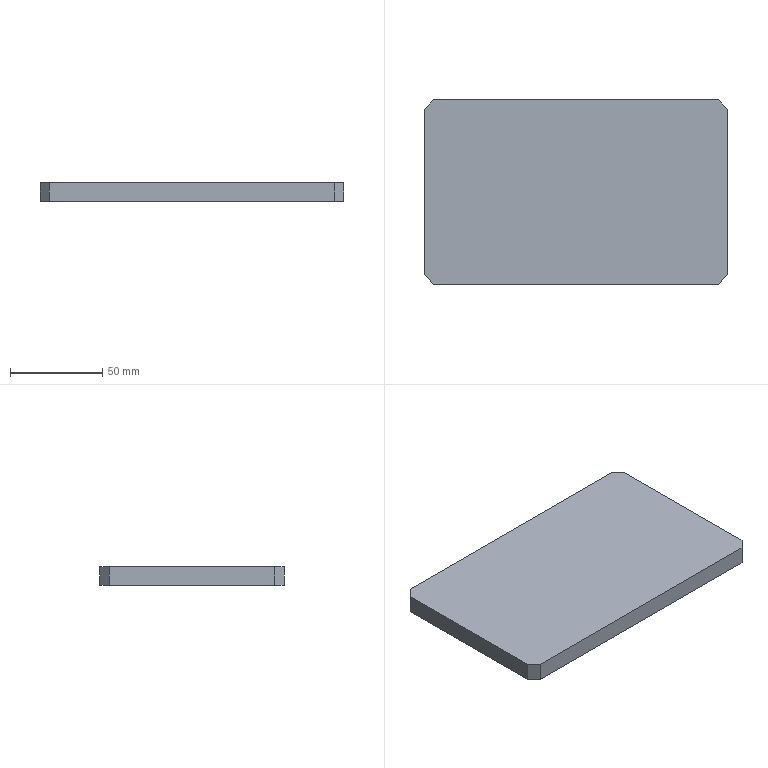Part | STEP file | Servo mount | 1 solid | 10 faces | box 165 x 100 x 10 mm | volume 164500 mm3 | plane 10
STEP:
#1=CARTESIAN_POINT('',(0.,0.,0.));
#2=DIRECTION('',(0.,0.,1.));
#3=DIRECTION('',(1.,0.,0.));
#4=AXIS2_PLACEMENT_3D('',#1,#2,#3);
#5=CARTESIAN_POINT('',(82.5,-45.,10.));
#6=VERTEX_POINT('',#5);
#7=CARTESIAN_POINT('',(82.5,45.,10.));
#8=VERTEX_POINT('',#7);
#9=CARTESIAN_POINT('',(82.5,50.,10.));
#10=DIRECTION('',(0.,1.,0.));
#11=VECTOR('',#10,1.);
#12=LINE('',#9,#11);
#13=CARTESIAN_POINT('',(82.5,50.,10.));
#14=DIRECTION('',(-1.,0.,0.));
#15=DIRECTION('',(0.,-1.,0.));
#16=AXIS2_PLACEMENT_3D('',#13,#14,#15);
#17=PLANE('',#16);
#18=CARTESIAN_POINT('',(0.,0.));
#19=DIRECTION('',(-1.,0.));
#20=VECTOR('',#19,1.);
#21=LINE('',#18,#20);
#22=(GEOMETRIC_REPRESENTATION_CONTEXT(2)PARAMETRIC_REPRESENTATION_CONTEXT()REPRESENTATION_CONTEXT('',''));
#23=DEFINITIONAL_REPRESENTATION('',(#21),#22);
#24=PCURVE('',#17,#23);
#25=CARTESIAN_POINT('',(82.5,-50.,10.));
#26=DIRECTION('',(0.,0.,1.));
#27=DIRECTION('',(1.,0.,0.));
#28=AXIS2_PLACEMENT_3D('',#25,#26,#27);
#29=PLANE('',#28);
#30=CARTESIAN_POINT('',(0.,100.));
#31=DIRECTION('',(0.,1.));
#32=VECTOR('',#31,1.);
#33=LINE('',#30,#32);
#34=(GEOMETRIC_REPRESENTATION_CONTEXT(2)PARAMETRIC_REPRESENTATION_CONTEXT()REPRESENTATION_CONTEXT('',''));
#35=DEFINITIONAL_REPRESENTATION('',(#33),#34);
#36=PCURVE('',#29,#35);
#37=SURFACE_CURVE('',#12,(#24,#36),.PCURVE_S1.);
#38=EDGE_CURVE('',#6,#8,#37,.T.);
#39=ORIENTED_EDGE('',*,*,#38,.F.);
#40=CARTESIAN_POINT('',(82.5,-45.,0.));
#41=VERTEX_POINT('',#40);
#42=CARTESIAN_POINT('',(82.5,-45.,10.));
#43=DIRECTION('',(0.,0.,-1.));
#44=VECTOR('',#43,1.);
#45=LINE('',#42,#44);
#46=CARTESIAN_POINT('',(95.,0.));
#47=DIRECTION('',(0.,-1.));
#48=VECTOR('',#47,1.);
#49=LINE('',#46,#48);
#50=(GEOMETRIC_REPRESENTATION_CONTEXT(2)PARAMETRIC_REPRESENTATION_CONTEXT()REPRESENTATION_CONTEXT('',''));
#51=DEFINITIONAL_REPRESENTATION('',(#49),#50);
#52=PCURVE('',#17,#51);
#53=CARTESIAN_POINT('',(82.5,-45.,10.));
#54=DIRECTION('',(-0.7071,0.7071,0.));
#55=DIRECTION('',(-0.7071,-0.7071,0.));
#56=AXIS2_PLACEMENT_3D('',#53,#54,#55);
#57=PLANE('',#56);
#58=CARTESIAN_POINT('',(0.,0.));
#59=DIRECTION('',(0.,-1.));
#60=VECTOR('',#59,1.);
#61=LINE('',#58,#60);
#62=(GEOMETRIC_REPRESENTATION_CONTEXT(2)PARAMETRIC_REPRESENTATION_CONTEXT()REPRESENTATION_CONTEXT('',''));
#63=DEFINITIONAL_REPRESENTATION('',(#61),#62);
#64=PCURVE('',#57,#63);
#65=SURFACE_CURVE('',#45,(#52,#64),.PCURVE_S1.);
#66=EDGE_CURVE('',#6,#41,#65,.T.);
#67=ORIENTED_EDGE('',*,*,#66,.T.);
#68=CARTESIAN_POINT('',(82.5,45.,0.));
#69=VERTEX_POINT('',#68);
#70=CARTESIAN_POINT('',(82.5,50.,0.));
#71=DIRECTION('',(0.,1.,0.));
#72=VECTOR('',#71,1.);
#73=LINE('',#70,#72);
#74=CARTESIAN_POINT('',(0.,-10.));
#75=DIRECTION('',(-1.,0.));
#76=VECTOR('',#75,1.);
#77=LINE('',#74,#76);
#78=(GEOMETRIC_REPRESENTATION_CONTEXT(2)PARAMETRIC_REPRESENTATION_CONTEXT()REPRESENTATION_CONTEXT('',''));
#79=DEFINITIONAL_REPRESENTATION('',(#77),#78);
#80=PCURVE('',#17,#79);
#81=CARTESIAN_POINT('',(82.5,-50.,0.));
#82=DIRECTION('',(0.,0.,1.));
#83=DIRECTION('',(1.,0.,0.));
#84=AXIS2_PLACEMENT_3D('',#81,#82,#83);
#85=PLANE('',#84);
#86=CARTESIAN_POINT('',(0.,100.));
#87=DIRECTION('',(0.,1.));
#88=VECTOR('',#87,1.);
#89=LINE('',#86,#88);
#90=(GEOMETRIC_REPRESENTATION_CONTEXT(2)PARAMETRIC_REPRESENTATION_CONTEXT()REPRESENTATION_CONTEXT('',''));
#91=DEFINITIONAL_REPRESENTATION('',(#89),#90);
#92=PCURVE('',#85,#91);
#93=SURFACE_CURVE('',#73,(#80,#92),.PCURVE_S1.);
#94=EDGE_CURVE('',#41,#69,#93,.T.);
#95=ORIENTED_EDGE('',*,*,#94,.T.);
#96=CARTESIAN_POINT('',(82.5,45.,10.));
#97=DIRECTION('',(0.,0.,1.));
#98=VECTOR('',#97,1.);
#99=LINE('',#96,#98);
#100=CARTESIAN_POINT('',(5.,0.));
#101=DIRECTION('',(0.,1.));
#102=VECTOR('',#101,1.);
#103=LINE('',#100,#102);
#104=(GEOMETRIC_REPRESENTATION_CONTEXT(2)PARAMETRIC_REPRESENTATION_CONTEXT()REPRESENTATION_CONTEXT('',''));
#105=DEFINITIONAL_REPRESENTATION('',(#103),#104);
#106=PCURVE('',#17,#105);
#107=CARTESIAN_POINT('',(77.5,50.,10.));
#108=DIRECTION('',(-0.7071,-0.7071,0.));
#109=DIRECTION('',(0.7071,-0.7071,0.));
#110=AXIS2_PLACEMENT_3D('',#107,#108,#109);
#111=PLANE('',#110);
#112=CARTESIAN_POINT('',(7.071,0.));
#113=DIRECTION('',(0.,1.));
#114=VECTOR('',#113,1.);
#115=LINE('',#112,#114);
#116=(GEOMETRIC_REPRESENTATION_CONTEXT(2)PARAMETRIC_REPRESENTATION_CONTEXT()REPRESENTATION_CONTEXT('',''));
#117=DEFINITIONAL_REPRESENTATION('',(#115),#116);
#118=PCURVE('',#111,#117);
#119=SURFACE_CURVE('',#99,(#106,#118),.PCURVE_S1.);
#120=EDGE_CURVE('',#69,#8,#119,.T.);
#121=ORIENTED_EDGE('',*,*,#120,.T.);
#122=EDGE_LOOP('',(#39,#67,#95,#121));
#123=FACE_BOUND('',#122,.T.);
#124=ADVANCED_FACE('',(#123),#17,.F.);
#125=CARTESIAN_POINT('',(77.5,50.,0.));
#126=VERTEX_POINT('',#125);
#127=CARTESIAN_POINT('',(-77.5,50.,0.));
#128=VERTEX_POINT('',#127);
#129=CARTESIAN_POINT('',(-82.5,50.,0.));
#130=DIRECTION('',(-1.,0.,0.));
#131=VECTOR('',#130,1.);
#132=LINE('',#129,#131);
#133=CARTESIAN_POINT('',(-82.5,50.,10.));
#134=DIRECTION('',(0.,-1.,0.));
#135=DIRECTION('',(0.,0.,-1.));
#136=AXIS2_PLACEMENT_3D('',#133,#134,#135);
#137=PLANE('',#136);
#138=CARTESIAN_POINT('',(10.,0.));
#139=DIRECTION('',(0.,-1.));
#140=VECTOR('',#139,1.);
#141=LINE('',#138,#140);
#142=(GEOMETRIC_REPRESENTATION_CONTEXT(2)PARAMETRIC_REPRESENTATION_CONTEXT()REPRESENTATION_CONTEXT('',''));
#143=DEFINITIONAL_REPRESENTATION('',(#141),#142);
#144=PCURVE('',#137,#143);
#145=CARTESIAN_POINT('',(-165.,100.));
#146=DIRECTION('',(-1.,0.));
#147=VECTOR('',#146,1.);
#148=LINE('',#145,#147);
#149=(GEOMETRIC_REPRESENTATION_CONTEXT(2)PARAMETRIC_REPRESENTATION_CONTEXT()REPRESENTATION_CONTEXT('',''));
#150=DEFINITIONAL_REPRESENTATION('',(#148),#149);
#151=PCURVE('',#85,#150);
#152=SURFACE_CURVE('',#132,(#144,#151),.PCURVE_S1.);
#153=EDGE_CURVE('',#126,#128,#152,.T.);
#154=ORIENTED_EDGE('',*,*,#153,.T.);
#155=CARTESIAN_POINT('',(-77.5,50.,10.));
#156=VERTEX_POINT('',#155);
#157=CARTESIAN_POINT('',(-77.5,50.,10.));
#158=DIRECTION('',(0.,0.,1.));
#159=VECTOR('',#158,1.);
#160=LINE('',#157,#159);
#161=CARTESIAN_POINT('',(0.,5.));
#162=DIRECTION('',(-1.,0.));
#163=VECTOR('',#162,1.);
#164=LINE('',#161,#163);
#165=(GEOMETRIC_REPRESENTATION_CONTEXT(2)PARAMETRIC_REPRESENTATION_CONTEXT()REPRESENTATION_CONTEXT('',''));
#166=DEFINITIONAL_REPRESENTATION('',(#164),#165);
#167=PCURVE('',#137,#166);
#168=CARTESIAN_POINT('',(-82.5,45.,10.));
#169=DIRECTION('',(0.7071,-0.7071,0.));
#170=DIRECTION('',(0.7071,0.7071,0.));
#171=AXIS2_PLACEMENT_3D('',#168,#169,#170);
#172=PLANE('',#171);
#173=CARTESIAN_POINT('',(7.071,0.));
#174=DIRECTION('',(0.,1.));
#175=VECTOR('',#174,1.);
#176=LINE('',#173,#175);
#177=(GEOMETRIC_REPRESENTATION_CONTEXT(2)PARAMETRIC_REPRESENTATION_CONTEXT()REPRESENTATION_CONTEXT('',''));
#178=DEFINITIONAL_REPRESENTATION('',(#176),#177);
#179=PCURVE('',#172,#178);
#180=SURFACE_CURVE('',#160,(#167,#179),.PCURVE_S1.);
#181=EDGE_CURVE('',#128,#156,#180,.T.);
#182=ORIENTED_EDGE('',*,*,#181,.T.);
#183=CARTESIAN_POINT('',(77.5,50.,10.));
#184=VERTEX_POINT('',#183);
#185=CARTESIAN_POINT('',(-82.5,50.,10.));
#186=DIRECTION('',(-1.,0.,0.));
#187=VECTOR('',#186,1.);
#188=LINE('',#185,#187);
#189=CARTESIAN_POINT('',(0.,0.));
#190=DIRECTION('',(0.,-1.));
#191=VECTOR('',#190,1.);
#192=LINE('',#189,#191);
#193=(GEOMETRIC_REPRESENTATION_CONTEXT(2)PARAMETRIC_REPRESENTATION_CONTEXT()REPRESENTATION_CONTEXT('',''));
#194=DEFINITIONAL_REPRESENTATION('',(#192),#193);
#195=PCURVE('',#137,#194);
#196=CARTESIAN_POINT('',(-165.,100.));
#197=DIRECTION('',(-1.,0.));
#198=VECTOR('',#197,1.);
#199=LINE('',#196,#198);
#200=(GEOMETRIC_REPRESENTATION_CONTEXT(2)PARAMETRIC_REPRESENTATION_CONTEXT()REPRESENTATION_CONTEXT('',''));
#201=DEFINITIONAL_REPRESENTATION('',(#199),#200);
#202=PCURVE('',#29,#201);
#203=SURFACE_CURVE('',#188,(#195,#202),.PCURVE_S1.);
#204=EDGE_CURVE('',#184,#156,#203,.T.);
#205=ORIENTED_EDGE('',*,*,#204,.F.);
#206=CARTESIAN_POINT('',(77.5,50.,10.));
#207=DIRECTION('',(0.,0.,-1.));
#208=VECTOR('',#207,1.);
#209=LINE('',#206,#208);
#210=CARTESIAN_POINT('',(0.,160.));
#211=DIRECTION('',(1.,0.));
#212=VECTOR('',#211,1.);
#213=LINE('',#210,#212);
#214=(GEOMETRIC_REPRESENTATION_CONTEXT(2)PARAMETRIC_REPRESENTATION_CONTEXT()REPRESENTATION_CONTEXT('',''));
#215=DEFINITIONAL_REPRESENTATION('',(#213),#214);
#216=PCURVE('',#137,#215);
#217=CARTESIAN_POINT('',(0.,0.));
#218=DIRECTION('',(0.,-1.));
#219=VECTOR('',#218,1.);
#220=LINE('',#217,#219);
#221=(GEOMETRIC_REPRESENTATION_CONTEXT(2)PARAMETRIC_REPRESENTATION_CONTEXT()REPRESENTATION_CONTEXT('',''));
#222=DEFINITIONAL_REPRESENTATION('',(#220),#221);
#223=PCURVE('',#111,#222);
#224=SURFACE_CURVE('',#209,(#216,#223),.PCURVE_S1.);
#225=EDGE_CURVE('',#184,#126,#224,.T.);
#226=ORIENTED_EDGE('',*,*,#225,.T.);
#227=EDGE_LOOP('',(#154,#182,#205,#226));
#228=FACE_BOUND('',#227,.T.);
#229=ADVANCED_FACE('',(#228),#137,.F.);
#230=CARTESIAN_POINT('',(-82.5,45.,10.));
#231=VERTEX_POINT('',#230);
#232=CARTESIAN_POINT('',(-82.5,-45.,10.));
#233=VERTEX_POINT('',#232);
#234=CARTESIAN_POINT('',(-82.5,50.,10.));
#235=DIRECTION('',(0.,-1.,0.));
#236=VECTOR('',#235,1.);
#237=LINE('',#234,#236);
#238=CARTESIAN_POINT('',(-82.5,50.,10.));
#239=DIRECTION('',(1.,0.,0.));
#240=DIRECTION('',(0.,1.,0.));
#241=AXIS2_PLACEMENT_3D('',#238,#239,#240);
#242=PLANE('',#241);
#243=CARTESIAN_POINT('',(0.,0.));
#244=DIRECTION('',(-1.,0.));
#245=VECTOR('',#244,1.);
#246=LINE('',#243,#245);
#247=(GEOMETRIC_REPRESENTATION_CONTEXT(2)PARAMETRIC_REPRESENTATION_CONTEXT()REPRESENTATION_CONTEXT('',''));
#248=DEFINITIONAL_REPRESENTATION('',(#246),#247);
#249=PCURVE('',#242,#248);
#250=CARTESIAN_POINT('',(-165.,100.));
#251=DIRECTION('',(0.,-1.));
#252=VECTOR('',#251,1.);
#253=LINE('',#250,#252);
#254=(GEOMETRIC_REPRESENTATION_CONTEXT(2)PARAMETRIC_REPRESENTATION_CONTEXT()REPRESENTATION_CONTEXT('',''));
#255=DEFINITIONAL_REPRESENTATION('',(#253),#254);
#256=PCURVE('',#29,#255);
#257=SURFACE_CURVE('',#237,(#249,#256),.PCURVE_S1.);
#258=EDGE_CURVE('',#231,#233,#257,.T.);
#259=ORIENTED_EDGE('',*,*,#258,.F.);
#260=CARTESIAN_POINT('',(-82.5,45.,0.));
#261=VERTEX_POINT('',#260);
#262=CARTESIAN_POINT('',(-82.5,45.,10.));
#263=DIRECTION('',(0.,0.,-1.));
#264=VECTOR('',#263,1.);
#265=LINE('',#262,#264);
#266=CARTESIAN_POINT('',(-5.,0.));
#267=DIRECTION('',(0.,-1.));
#268=VECTOR('',#267,1.);
#269=LINE('',#266,#268);
#270=(GEOMETRIC_REPRESENTATION_CONTEXT(2)PARAMETRIC_REPRESENTATION_CONTEXT()REPRESENTATION_CONTEXT('',''));
#271=DEFINITIONAL_REPRESENTATION('',(#269),#270);
#272=PCURVE('',#242,#271);
#273=CARTESIAN_POINT('',(0.,0.));
#274=DIRECTION('',(0.,-1.));
#275=VECTOR('',#274,1.);
#276=LINE('',#273,#275);
#277=(GEOMETRIC_REPRESENTATION_CONTEXT(2)PARAMETRIC_REPRESENTATION_CONTEXT()REPRESENTATION_CONTEXT('',''));
#278=DEFINITIONAL_REPRESENTATION('',(#276),#277);
#279=PCURVE('',#172,#278);
#280=SURFACE_CURVE('',#265,(#272,#279),.PCURVE_S1.);
#281=EDGE_CURVE('',#231,#261,#280,.T.);
#282=ORIENTED_EDGE('',*,*,#281,.T.);
#283=CARTESIAN_POINT('',(-82.5,-45.,0.));
#284=VERTEX_POINT('',#283);
#285=CARTESIAN_POINT('',(-82.5,50.,0.));
#286=DIRECTION('',(0.,-1.,0.));
#287=VECTOR('',#286,1.);
#288=LINE('',#285,#287);
#289=CARTESIAN_POINT('',(0.,-10.));
#290=DIRECTION('',(-1.,0.));
#291=VECTOR('',#290,1.);
#292=LINE('',#289,#291);
#293=(GEOMETRIC_REPRESENTATION_CONTEXT(2)PARAMETRIC_REPRESENTATION_CONTEXT()REPRESENTATION_CONTEXT('',''));
#294=DEFINITIONAL_REPRESENTATION('',(#292),#293);
#295=PCURVE('',#242,#294);
#296=CARTESIAN_POINT('',(-165.,100.));
#297=DIRECTION('',(0.,-1.));
#298=VECTOR('',#297,1.);
#299=LINE('',#296,#298);
#300=(GEOMETRIC_REPRESENTATION_CONTEXT(2)PARAMETRIC_REPRESENTATION_CONTEXT()REPRESENTATION_CONTEXT('',''));
#301=DEFINITIONAL_REPRESENTATION('',(#299),#300);
#302=PCURVE('',#85,#301);
#303=SURFACE_CURVE('',#288,(#295,#302),.PCURVE_S1.);
#304=EDGE_CURVE('',#261,#284,#303,.T.);
#305=ORIENTED_EDGE('',*,*,#304,.T.);
#306=CARTESIAN_POINT('',(-82.5,-45.,10.));
#307=DIRECTION('',(0.,0.,1.));
#308=VECTOR('',#307,1.);
#309=LINE('',#306,#308);
#310=CARTESIAN_POINT('',(-95.,0.));
#311=DIRECTION('',(0.,1.));
#312=VECTOR('',#311,1.);
#313=LINE('',#310,#312);
#314=(GEOMETRIC_REPRESENTATION_CONTEXT(2)PARAMETRIC_REPRESENTATION_CONTEXT()REPRESENTATION_CONTEXT('',''));
#315=DEFINITIONAL_REPRESENTATION('',(#313),#314);
#316=PCURVE('',#242,#315);
#317=CARTESIAN_POINT('',(-77.5,-50.,10.));
#318=DIRECTION('',(0.7071,0.7071,0.));
#319=DIRECTION('',(-0.7071,0.7071,0.));
#320=AXIS2_PLACEMENT_3D('',#317,#318,#319);
#321=PLANE('',#320);
#322=CARTESIAN_POINT('',(7.071,0.));
#323=DIRECTION('',(0.,1.));
#324=VECTOR('',#323,1.);
#325=LINE('',#322,#324);
#326=(GEOMETRIC_REPRESENTATION_CONTEXT(2)PARAMETRIC_REPRESENTATION_CONTEXT()REPRESENTATION_CONTEXT('',''));
#327=DEFINITIONAL_REPRESENTATION('',(#325),#326);
#328=PCURVE('',#321,#327);
#329=SURFACE_CURVE('',#309,(#316,#328),.PCURVE_S1.);
#330=EDGE_CURVE('',#284,#233,#329,.T.);
#331=ORIENTED_EDGE('',*,*,#330,.T.);
#332=EDGE_LOOP('',(#259,#282,#305,#331));
#333=FACE_BOUND('',#332,.T.);
#334=ADVANCED_FACE('',(#333),#242,.F.);
#335=CARTESIAN_POINT('',(-77.5,-50.,10.));
#336=VERTEX_POINT('',#335);
#337=CARTESIAN_POINT('',(77.5,-50.,10.));
#338=VERTEX_POINT('',#337);
#339=CARTESIAN_POINT('',(-82.5,-50.,10.));
#340=DIRECTION('',(1.,0.,0.));
#341=VECTOR('',#340,1.);
#342=LINE('',#339,#341);
#343=CARTESIAN_POINT('',(-82.5,-50.,10.));
#344=DIRECTION('',(0.,1.,0.));
#345=DIRECTION('',(0.,0.,1.));
#346=AXIS2_PLACEMENT_3D('',#343,#344,#345);
#347=PLANE('',#346);
#348=CARTESIAN_POINT('',(0.,0.));
#349=DIRECTION('',(0.,1.));
#350=VECTOR('',#349,1.);
#351=LINE('',#348,#350);
#352=(GEOMETRIC_REPRESENTATION_CONTEXT(2)PARAMETRIC_REPRESENTATION_CONTEXT()REPRESENTATION_CONTEXT('',''));
#353=DEFINITIONAL_REPRESENTATION('',(#351),#352);
#354=PCURVE('',#347,#353);
#355=CARTESIAN_POINT('',(-165.,0.));
#356=DIRECTION('',(1.,0.));
#357=VECTOR('',#356,1.);
#358=LINE('',#355,#357);
#359=(GEOMETRIC_REPRESENTATION_CONTEXT(2)PARAMETRIC_REPRESENTATION_CONTEXT()REPRESENTATION_CONTEXT('',''));
#360=DEFINITIONAL_REPRESENTATION('',(#358),#359);
#361=PCURVE('',#29,#360);
#362=SURFACE_CURVE('',#342,(#354,#361),.PCURVE_S1.);
#363=EDGE_CURVE('',#336,#338,#362,.T.);
#364=ORIENTED_EDGE('',*,*,#363,.F.);
#365=CARTESIAN_POINT('',(-77.5,-50.,0.));
#366=VERTEX_POINT('',#365);
#367=CARTESIAN_POINT('',(-77.5,-50.,10.));
#368=DIRECTION('',(0.,0.,-1.));
#369=VECTOR('',#368,1.);
#370=LINE('',#367,#369);
#371=CARTESIAN_POINT('',(0.,5.));
#372=DIRECTION('',(-1.,0.));
#373=VECTOR('',#372,1.);
#374=LINE('',#371,#373);
#375=(GEOMETRIC_REPRESENTATION_CONTEXT(2)PARAMETRIC_REPRESENTATION_CONTEXT()REPRESENTATION_CONTEXT('',''));
#376=DEFINITIONAL_REPRESENTATION('',(#374),#375);
#377=PCURVE('',#347,#376);
#378=CARTESIAN_POINT('',(0.,0.));
#379=DIRECTION('',(0.,-1.));
#380=VECTOR('',#379,1.);
#381=LINE('',#378,#380);
#382=(GEOMETRIC_REPRESENTATION_CONTEXT(2)PARAMETRIC_REPRESENTATION_CONTEXT()REPRESENTATION_CONTEXT('',''));
#383=DEFINITIONAL_REPRESENTATION('',(#381),#382);
#384=PCURVE('',#321,#383);
#385=SURFACE_CURVE('',#370,(#377,#384),.PCURVE_S1.);
#386=EDGE_CURVE('',#336,#366,#385,.T.);
#387=ORIENTED_EDGE('',*,*,#386,.T.);
#388=CARTESIAN_POINT('',(77.5,-50.,0.));
#389=VERTEX_POINT('',#388);
#390=CARTESIAN_POINT('',(-82.5,-50.,0.));
#391=DIRECTION('',(1.,0.,0.));
#392=VECTOR('',#391,1.);
#393=LINE('',#390,#392);
#394=CARTESIAN_POINT('',(-10.,0.));
#395=DIRECTION('',(0.,1.));
#396=VECTOR('',#395,1.);
#397=LINE('',#394,#396);
#398=(GEOMETRIC_REPRESENTATION_CONTEXT(2)PARAMETRIC_REPRESENTATION_CONTEXT()REPRESENTATION_CONTEXT('',''));
#399=DEFINITIONAL_REPRESENTATION('',(#397),#398);
#400=PCURVE('',#347,#399);
#401=CARTESIAN_POINT('',(-165.,0.));
#402=DIRECTION('',(1.,0.));
#403=VECTOR('',#402,1.);
#404=LINE('',#401,#403);
#405=(GEOMETRIC_REPRESENTATION_CONTEXT(2)PARAMETRIC_REPRESENTATION_CONTEXT()REPRESENTATION_CONTEXT('',''));
#406=DEFINITIONAL_REPRESENTATION('',(#404),#405);
#407=PCURVE('',#85,#406);
#408=SURFACE_CURVE('',#393,(#400,#407),.PCURVE_S1.);
#409=EDGE_CURVE('',#366,#389,#408,.T.);
#410=ORIENTED_EDGE('',*,*,#409,.T.);
#411=CARTESIAN_POINT('',(77.5,-50.,10.));
#412=DIRECTION('',(0.,0.,1.));
#413=VECTOR('',#412,1.);
#414=LINE('',#411,#413);
#415=CARTESIAN_POINT('',(0.,160.));
#416=DIRECTION('',(1.,0.));
#417=VECTOR('',#416,1.);
#418=LINE('',#415,#417);
#419=(GEOMETRIC_REPRESENTATION_CONTEXT(2)PARAMETRIC_REPRESENTATION_CONTEXT()REPRESENTATION_CONTEXT('',''));
#420=DEFINITIONAL_REPRESENTATION('',(#418),#419);
#421=PCURVE('',#347,#420);
#422=CARTESIAN_POINT('',(7.071,0.));
#423=DIRECTION('',(0.,1.));
#424=VECTOR('',#423,1.);
#425=LINE('',#422,#424);
#426=(GEOMETRIC_REPRESENTATION_CONTEXT(2)PARAMETRIC_REPRESENTATION_CONTEXT()REPRESENTATION_CONTEXT('',''));
#427=DEFINITIONAL_REPRESENTATION('',(#425),#426);
#428=PCURVE('',#57,#427);
#429=SURFACE_CURVE('',#414,(#421,#428),.PCURVE_S1.);
#430=EDGE_CURVE('',#389,#338,#429,.T.);
#431=ORIENTED_EDGE('',*,*,#430,.T.);
#432=EDGE_LOOP('',(#364,#387,#410,#431));
#433=FACE_BOUND('',#432,.T.);
#434=ADVANCED_FACE('',(#433),#347,.F.);
#435=ORIENTED_EDGE('',*,*,#204,.T.);
#436=CARTESIAN_POINT('',(-47.5,80.,10.));
#437=DIRECTION('',(-0.7071,-0.7071,0.));
#438=VECTOR('',#437,1.);
#439=LINE('',#436,#438);
#440=CARTESIAN_POINT('',(-130.,130.));
#441=DIRECTION('',(-0.7071,-0.7071));
#442=VECTOR('',#441,1.);
#443=LINE('',#440,#442);
#444=(GEOMETRIC_REPRESENTATION_CONTEXT(2)PARAMETRIC_REPRESENTATION_CONTEXT()REPRESENTATION_CONTEXT('',''));
#445=DEFINITIONAL_REPRESENTATION('',(#443),#444);
#446=PCURVE('',#29,#445);
#447=CARTESIAN_POINT('',(49.497,0.));
#448=DIRECTION('',(-1.,0.));
#449=VECTOR('',#448,1.);
#450=LINE('',#447,#449);
#451=(GEOMETRIC_REPRESENTATION_CONTEXT(2)PARAMETRIC_REPRESENTATION_CONTEXT()REPRESENTATION_CONTEXT('',''));
#452=DEFINITIONAL_REPRESENTATION('',(#450),#451);
#453=PCURVE('',#172,#452);
#454=SURFACE_CURVE('',#439,(#446,#453),.PCURVE_S1.);
#455=EDGE_CURVE('',#156,#231,#454,.T.);
#456=ORIENTED_EDGE('',*,*,#455,.T.);
#457=ORIENTED_EDGE('',*,*,#258,.T.);
#458=CARTESIAN_POINT('',(2.5,-130.,10.));
#459=DIRECTION('',(0.7071,-0.7071,0.));
#460=VECTOR('',#459,1.);
#461=LINE('',#458,#460);
#462=CARTESIAN_POINT('',(-80.,-80.));
#463=DIRECTION('',(0.7071,-0.7071));
#464=VECTOR('',#463,1.);
#465=LINE('',#462,#464);
#466=(GEOMETRIC_REPRESENTATION_CONTEXT(2)PARAMETRIC_REPRESENTATION_CONTEXT()REPRESENTATION_CONTEXT('',''));
#467=DEFINITIONAL_REPRESENTATION('',(#465),#466);
#468=PCURVE('',#29,#467);
#469=CARTESIAN_POINT('',(-113.137,0.));
#470=DIRECTION('',(-1.,0.));
#471=VECTOR('',#470,1.);
#472=LINE('',#469,#471);
#473=(GEOMETRIC_REPRESENTATION_CONTEXT(2)PARAMETRIC_REPRESENTATION_CONTEXT()REPRESENTATION_CONTEXT('',''));
#474=DEFINITIONAL_REPRESENTATION('',(#472),#473);
#475=PCURVE('',#321,#474);
#476=SURFACE_CURVE('',#461,(#468,#475),.PCURVE_S1.);
#477=EDGE_CURVE('',#233,#336,#476,.T.);
#478=ORIENTED_EDGE('',*,*,#477,.T.);
#479=ORIENTED_EDGE('',*,*,#363,.T.);
#480=CARTESIAN_POINT('',(80.,-47.5,10.));
#481=DIRECTION('',(0.7071,0.7071,0.));
#482=VECTOR('',#481,1.);
#483=LINE('',#480,#482);
#484=CARTESIAN_POINT('',(-2.5,2.5));
#485=DIRECTION('',(0.7071,0.7071));
#486=VECTOR('',#485,1.);
#487=LINE('',#484,#486);
#488=(GEOMETRIC_REPRESENTATION_CONTEXT(2)PARAMETRIC_REPRESENTATION_CONTEXT()REPRESENTATION_CONTEXT('',''));
#489=DEFINITIONAL_REPRESENTATION('',(#487),#488);
#490=PCURVE('',#29,#489);
#491=CARTESIAN_POINT('',(3.536,0.));
#492=DIRECTION('',(-1.,0.));
#493=VECTOR('',#492,1.);
#494=LINE('',#491,#493);
#495=(GEOMETRIC_REPRESENTATION_CONTEXT(2)PARAMETRIC_REPRESENTATION_CONTEXT()REPRESENTATION_CONTEXT('',''));
#496=DEFINITIONAL_REPRESENTATION('',(#494),#495);
#497=PCURVE('',#57,#496);
#498=SURFACE_CURVE('',#483,(#490,#497),.PCURVE_S1.);
#499=EDGE_CURVE('',#338,#6,#498,.T.);
#500=ORIENTED_EDGE('',*,*,#499,.T.);
#501=ORIENTED_EDGE('',*,*,#38,.T.);
#502=CARTESIAN_POINT('',(130.,-2.5,10.));
#503=DIRECTION('',(-0.7071,0.7071,0.));
#504=VECTOR('',#503,1.);
#505=LINE('',#502,#504);
#506=CARTESIAN_POINT('',(47.5,47.5));
#507=DIRECTION('',(-0.7071,0.7071));
#508=VECTOR('',#507,1.);
#509=LINE('',#506,#508);
#510=(GEOMETRIC_REPRESENTATION_CONTEXT(2)PARAMETRIC_REPRESENTATION_CONTEXT()REPRESENTATION_CONTEXT('',''));
#511=DEFINITIONAL_REPRESENTATION('',(#509),#510);
#512=PCURVE('',#29,#511);
#513=CARTESIAN_POINT('',(74.246,0.));
#514=DIRECTION('',(-1.,0.));
#515=VECTOR('',#514,1.);
#516=LINE('',#513,#515);
#517=(GEOMETRIC_REPRESENTATION_CONTEXT(2)PARAMETRIC_REPRESENTATION_CONTEXT()REPRESENTATION_CONTEXT('',''));
#518=DEFINITIONAL_REPRESENTATION('',(#516),#517);
#519=PCURVE('',#111,#518);
#520=SURFACE_CURVE('',#505,(#512,#519),.PCURVE_S1.);
#521=EDGE_CURVE('',#8,#184,#520,.T.);
#522=ORIENTED_EDGE('',*,*,#521,.T.);
#523=EDGE_LOOP('',(#435,#456,#457,#478,#479,#500,#501,#522));
#524=FACE_BOUND('',#523,.T.);
#525=ADVANCED_FACE('',(#524),#29,.T.);
#526=ORIENTED_EDGE('',*,*,#304,.F.);
#527=CARTESIAN_POINT('',(-82.5,45.,0.));
#528=DIRECTION('',(0.7071,0.7071,0.));
#529=VECTOR('',#528,1.);
#530=LINE('',#527,#529);
#531=CARTESIAN_POINT('',(-165.,95.));
#532=DIRECTION('',(0.7071,0.7071));
#533=VECTOR('',#532,1.);
#534=LINE('',#531,#533);
#535=(GEOMETRIC_REPRESENTATION_CONTEXT(2)PARAMETRIC_REPRESENTATION_CONTEXT()REPRESENTATION_CONTEXT('',''));
#536=DEFINITIONAL_REPRESENTATION('',(#534),#535);
#537=PCURVE('',#85,#536);
#538=CARTESIAN_POINT('',(0.,-10.));
#539=DIRECTION('',(1.,0.));
#540=VECTOR('',#539,1.);
#541=LINE('',#538,#540);
#542=(GEOMETRIC_REPRESENTATION_CONTEXT(2)PARAMETRIC_REPRESENTATION_CONTEXT()REPRESENTATION_CONTEXT('',''));
#543=DEFINITIONAL_REPRESENTATION('',(#541),#542);
#544=PCURVE('',#172,#543);
#545=SURFACE_CURVE('',#530,(#537,#544),.PCURVE_S1.);
#546=EDGE_CURVE('',#261,#128,#545,.T.);
#547=ORIENTED_EDGE('',*,*,#546,.T.);
#548=ORIENTED_EDGE('',*,*,#153,.F.);
#549=CARTESIAN_POINT('',(77.5,50.,0.));
#550=DIRECTION('',(0.7071,-0.7071,0.));
#551=VECTOR('',#550,1.);
#552=LINE('',#549,#551);
#553=CARTESIAN_POINT('',(-5.,100.));
#554=DIRECTION('',(0.7071,-0.7071));
#555=VECTOR('',#554,1.);
#556=LINE('',#553,#555);
#557=(GEOMETRIC_REPRESENTATION_CONTEXT(2)PARAMETRIC_REPRESENTATION_CONTEXT()REPRESENTATION_CONTEXT('',''));
#558=DEFINITIONAL_REPRESENTATION('',(#556),#557);
#559=PCURVE('',#85,#558);
#560=CARTESIAN_POINT('',(0.,-10.));
#561=DIRECTION('',(1.,0.));
#562=VECTOR('',#561,1.);
#563=LINE('',#560,#562);
#564=(GEOMETRIC_REPRESENTATION_CONTEXT(2)PARAMETRIC_REPRESENTATION_CONTEXT()REPRESENTATION_CONTEXT('',''));
#565=DEFINITIONAL_REPRESENTATION('',(#563),#564);
#566=PCURVE('',#111,#565);
#567=SURFACE_CURVE('',#552,(#559,#566),.PCURVE_S1.);
#568=EDGE_CURVE('',#126,#69,#567,.T.);
#569=ORIENTED_EDGE('',*,*,#568,.T.);
#570=ORIENTED_EDGE('',*,*,#94,.F.);
#571=CARTESIAN_POINT('',(82.5,-45.,0.));
#572=DIRECTION('',(-0.7071,-0.7071,0.));
#573=VECTOR('',#572,1.);
#574=LINE('',#571,#573);
#575=CARTESIAN_POINT('',(0.,5.));
#576=DIRECTION('',(-0.7071,-0.7071));
#577=VECTOR('',#576,1.);
#578=LINE('',#575,#577);
#579=(GEOMETRIC_REPRESENTATION_CONTEXT(2)PARAMETRIC_REPRESENTATION_CONTEXT()REPRESENTATION_CONTEXT('',''));
#580=DEFINITIONAL_REPRESENTATION('',(#578),#579);
#581=PCURVE('',#85,#580);
#582=CARTESIAN_POINT('',(0.,-10.));
#583=DIRECTION('',(1.,0.));
#584=VECTOR('',#583,1.);
#585=LINE('',#582,#584);
#586=(GEOMETRIC_REPRESENTATION_CONTEXT(2)PARAMETRIC_REPRESENTATION_CONTEXT()REPRESENTATION_CONTEXT('',''));
#587=DEFINITIONAL_REPRESENTATION('',(#585),#586);
#588=PCURVE('',#57,#587);
#589=SURFACE_CURVE('',#574,(#581,#588),.PCURVE_S1.);
#590=EDGE_CURVE('',#41,#389,#589,.T.);
#591=ORIENTED_EDGE('',*,*,#590,.T.);
#592=ORIENTED_EDGE('',*,*,#409,.F.);
#593=CARTESIAN_POINT('',(-77.5,-50.,0.));
#594=DIRECTION('',(-0.7071,0.7071,0.));
#595=VECTOR('',#594,1.);
#596=LINE('',#593,#595);
#597=CARTESIAN_POINT('',(-160.,0.));
#598=DIRECTION('',(-0.7071,0.7071));
#599=VECTOR('',#598,1.);
#600=LINE('',#597,#599);
#601=(GEOMETRIC_REPRESENTATION_CONTEXT(2)PARAMETRIC_REPRESENTATION_CONTEXT()REPRESENTATION_CONTEXT('',''));
#602=DEFINITIONAL_REPRESENTATION('',(#600),#601);
#603=PCURVE('',#85,#602);
#604=CARTESIAN_POINT('',(0.,-10.));
#605=DIRECTION('',(1.,0.));
#606=VECTOR('',#605,1.);
#607=LINE('',#604,#606);
#608=(GEOMETRIC_REPRESENTATION_CONTEXT(2)PARAMETRIC_REPRESENTATION_CONTEXT()REPRESENTATION_CONTEXT('',''));
#609=DEFINITIONAL_REPRESENTATION('',(#607),#608);
#610=PCURVE('',#321,#609);
#611=SURFACE_CURVE('',#596,(#603,#610),.PCURVE_S1.);
#612=EDGE_CURVE('',#366,#284,#611,.T.);
#613=ORIENTED_EDGE('',*,*,#612,.T.);
#614=EDGE_LOOP('',(#526,#547,#548,#569,#570,#591,#592,#613));
#615=FACE_BOUND('',#614,.T.);
#616=ADVANCED_FACE('',(#615),#85,.F.);
#617=ORIENTED_EDGE('',*,*,#455,.F.);
#618=ORIENTED_EDGE('',*,*,#181,.F.);
#619=ORIENTED_EDGE('',*,*,#546,.F.);
#620=ORIENTED_EDGE('',*,*,#281,.F.);
#621=EDGE_LOOP('',(#617,#618,#619,#620));
#622=FACE_BOUND('',#621,.T.);
#623=ADVANCED_FACE('',(#622),#172,.F.);
#624=ORIENTED_EDGE('',*,*,#477,.F.);
#625=ORIENTED_EDGE('',*,*,#330,.F.);
#626=ORIENTED_EDGE('',*,*,#612,.F.);
#627=ORIENTED_EDGE('',*,*,#386,.F.);
#628=EDGE_LOOP('',(#624,#625,#626,#627));
#629=FACE_BOUND('',#628,.T.);
#630=ADVANCED_FACE('',(#629),#321,.F.);
#631=ORIENTED_EDGE('',*,*,#499,.F.);
#632=ORIENTED_EDGE('',*,*,#430,.F.);
#633=ORIENTED_EDGE('',*,*,#590,.F.);
#634=ORIENTED_EDGE('',*,*,#66,.F.);
#635=EDGE_LOOP('',(#631,#632,#633,#634));
#636=FACE_BOUND('',#635,.T.);
#637=ADVANCED_FACE('',(#636),#57,.F.);
#638=ORIENTED_EDGE('',*,*,#521,.F.);
#639=ORIENTED_EDGE('',*,*,#120,.F.);
#640=ORIENTED_EDGE('',*,*,#568,.F.);
#641=ORIENTED_EDGE('',*,*,#225,.F.);
#642=EDGE_LOOP('',(#638,#639,#640,#641));
#643=FACE_BOUND('',#642,.T.);
#644=ADVANCED_FACE('',(#643),#111,.F.);
#645=CLOSED_SHELL('',(#124,#229,#334,#434,#525,#616,#623,#630,#637,#644));
#646=MANIFOLD_SOLID_BREP('',#645);
#647=(LENGTH_UNIT()NAMED_UNIT(*)SI_UNIT(.MILLI.,.METRE.));
#648=UNCERTAINTY_MEASURE_WITH_UNIT(LENGTH_MEASURE(0.0000001),#647,'','');
#649=(NAMED_UNIT(*)PLANE_ANGLE_UNIT()SI_UNIT($,.RADIAN.));
#650=(NAMED_UNIT(*)SI_UNIT($,.STERADIAN.)SOLID_ANGLE_UNIT());
#651=(GEOMETRIC_REPRESENTATION_CONTEXT(3)GLOBAL_UNCERTAINTY_ASSIGNED_CONTEXT((#648))GLOBAL_UNIT_ASSIGNED_CONTEXT((#647,#649,#650))REPRESENTATION_CONTEXT('',''));
#652=ADVANCED_BREP_SHAPE_REPRESENTATION('',(#4,#646),#651);